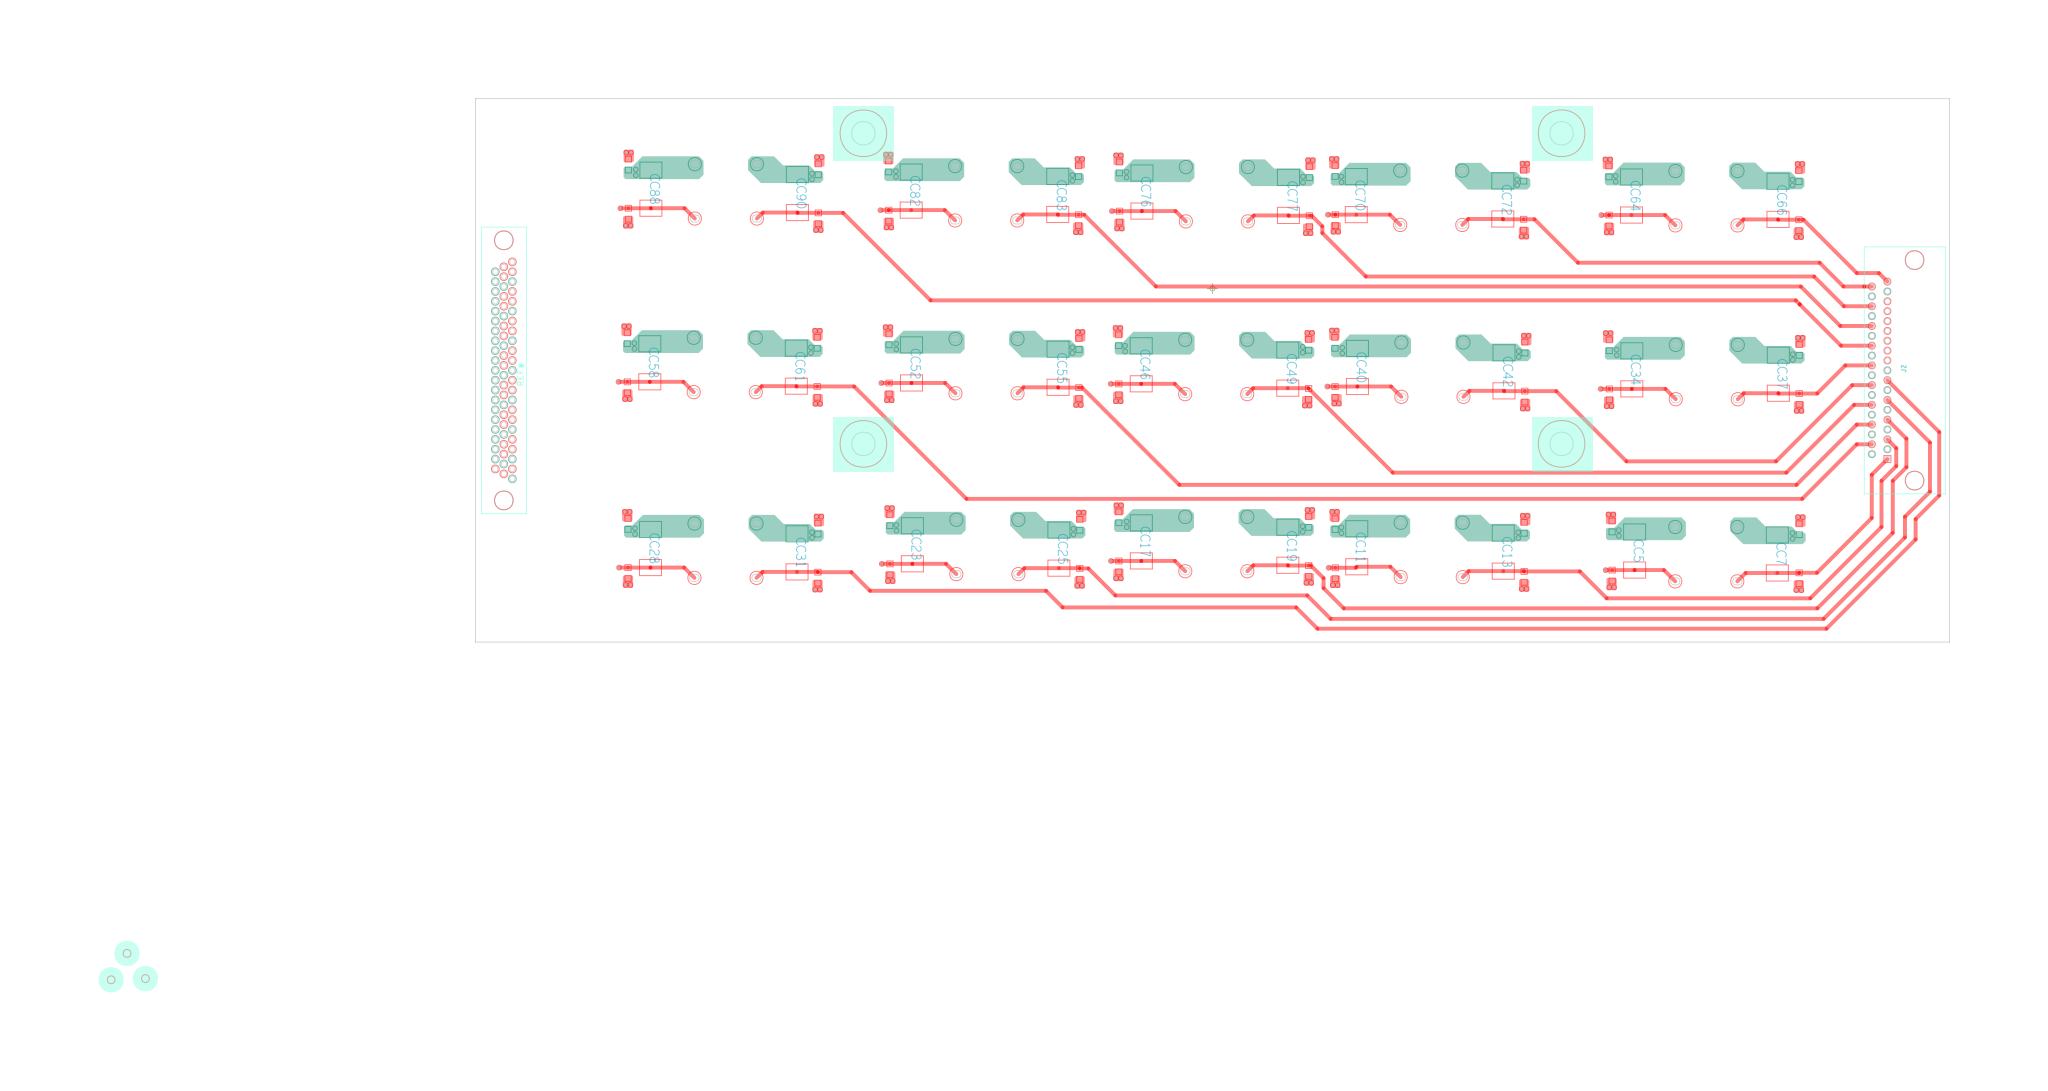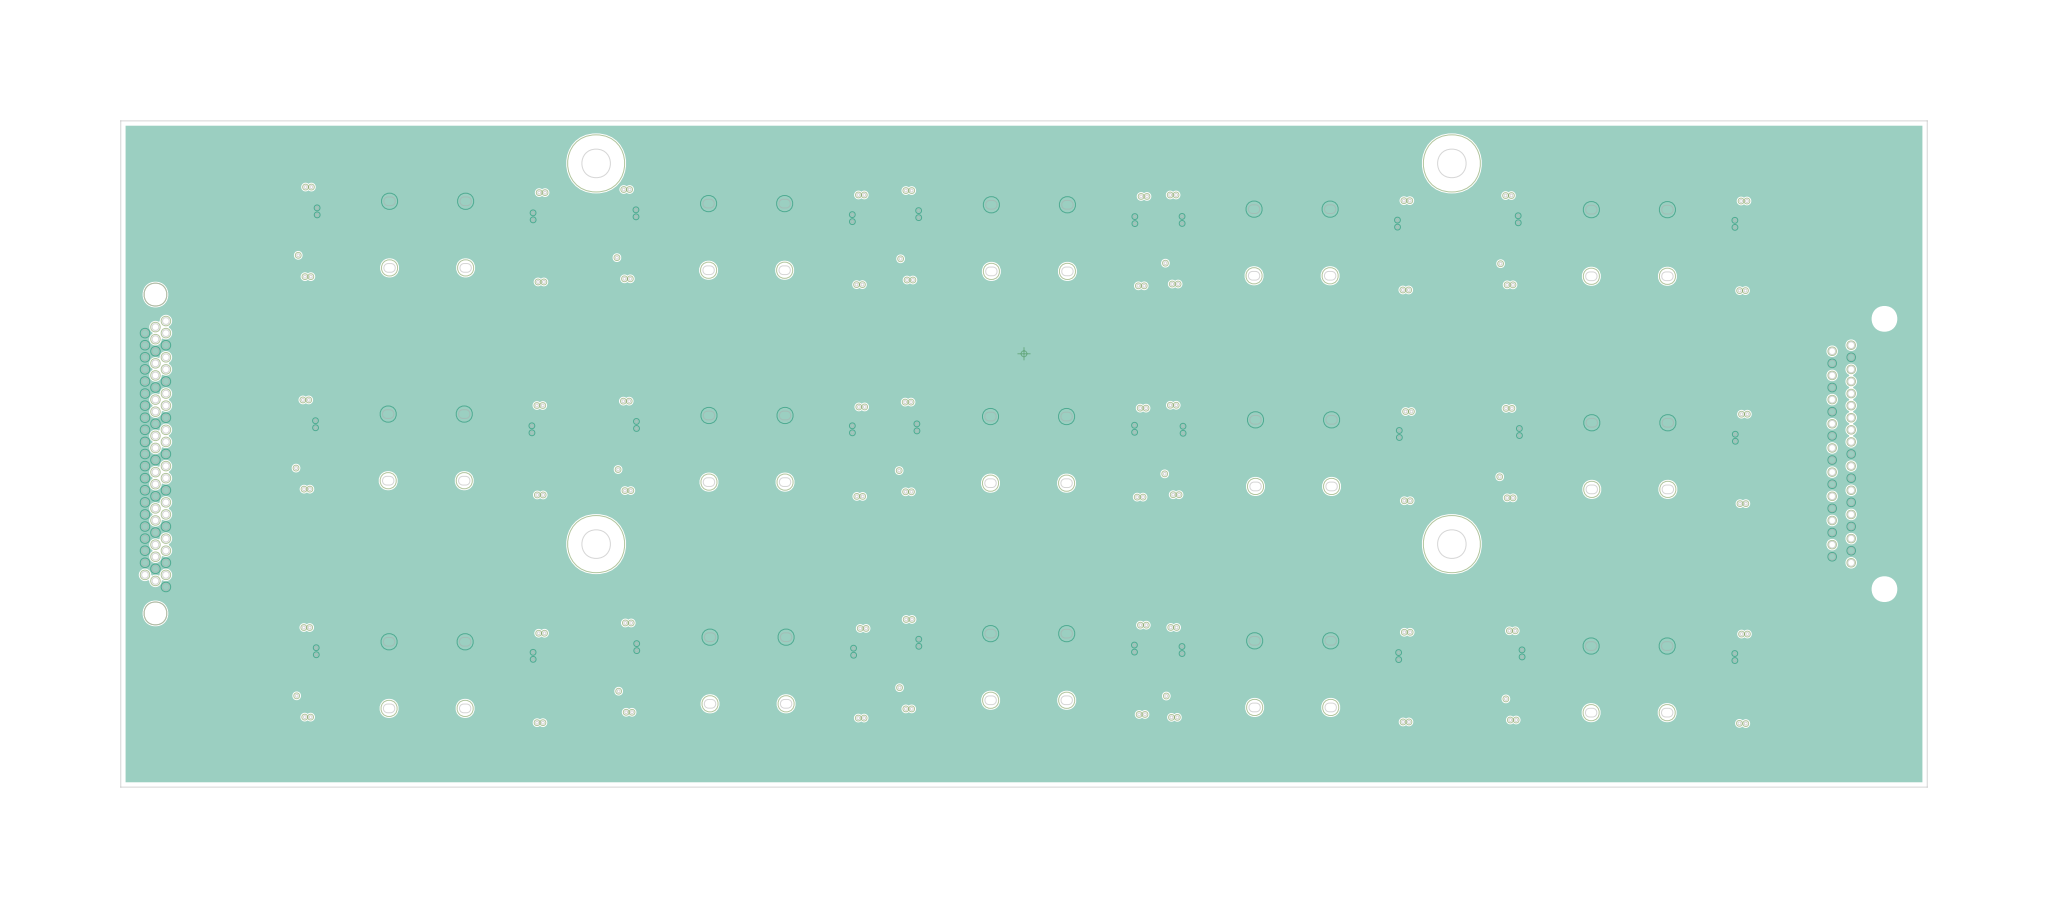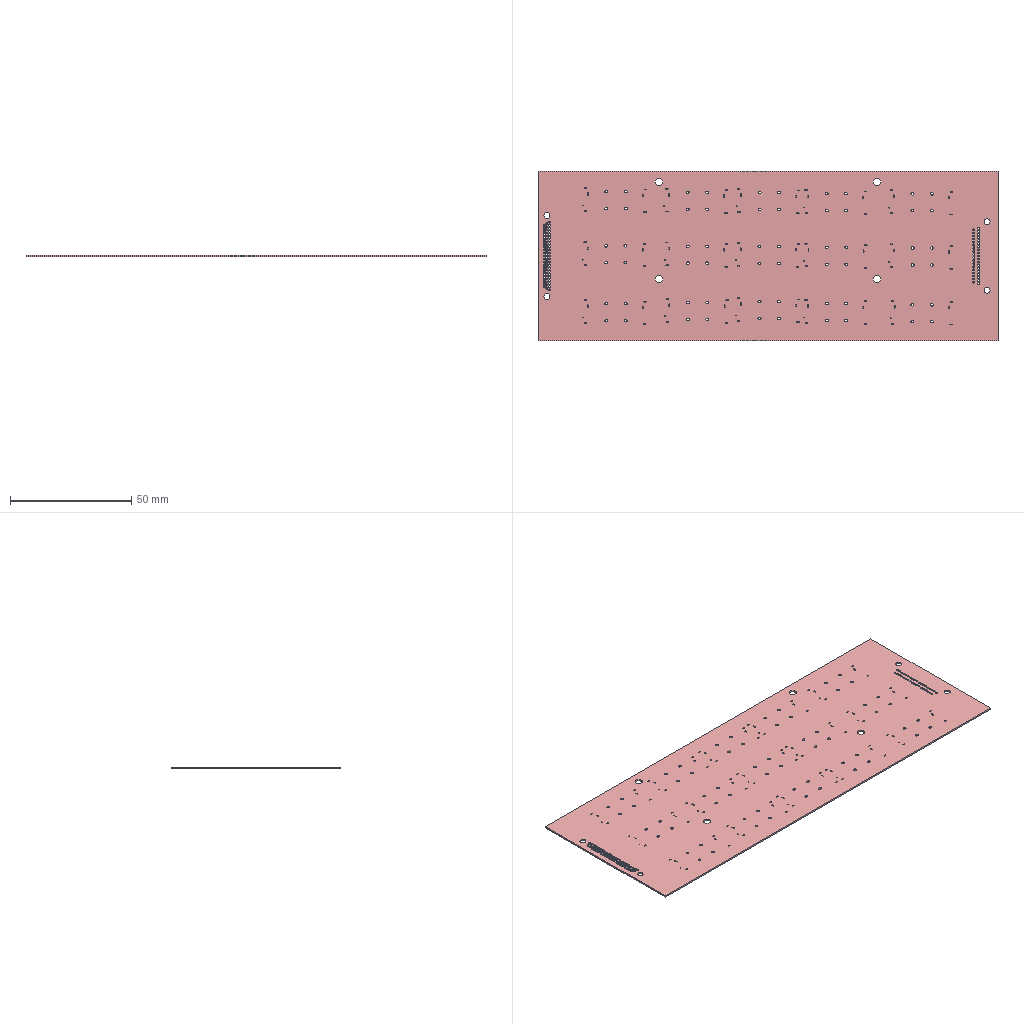Circuit board layout | Cadence Allegro | box 190 x 70 x 0.7 mm
Layer stack:
# Cadence Allegro layer stack of  (unit mm; from the constraint file cross-section; dielectric type: 0 not recorded (Allegro does not mark core vs prepreg), 3 surface material)
index,name,kind,layer,copper_thickness_mm,dielectric_type,dielectric_thickness_mm,dielectric_material,dielectric_constant
0,Top Surface,other,,,,,,
1,TOP,copper,TOP,0.0305,,,,
2,Dielectric1,dielectric,,,0,0.2032,FR-4,4.5
3,GND2,copper,GND2,0.0305,,,,
4,Dielectric2,dielectric,,,0,0.2032,FR-4,4.5
5,GND3,copper,GND3,0.0305,,,,
6,Dielectric3,dielectric,,,0,0.2032,FR-4,4.5
7,BOTTOM,copper,BOTTOM,0.0305,,,,
8,Bottom Surface,other,,,,,,
# drill layer pairs: low layer,high layer
drill_pair,TOP,BOTTOM
Part placement:
REFDES,COMP_VALUE,SYM_NAME,SYM_X,SYM_Y,SYM_ROTATE,SYM_MIRROR
CC4,1uF/50V,C0603,2027.992,-1206.161,270.000,NO
CC5,68uF/50V,C1812,2142.256,-1330.882,270.000,NO
CC6,1uF/50V,C0603,2028.386,-1455.201,270.000,NO
CC7,68uF/50V,C1812,2866.543,-1345.756,270.000,NO
CC8,1uF/50V,C0603,2977.339,-1468.843,270.000,NO
CC9,1uF/50V,C0603,2977.339,-1220.193,270.000,NO
CC10,1uF/50V,C0603,622.668,-1194.281,270.000,NO
CC11,68uF/50V,C1812,732.112,-1314.185,270.000,NO
CC12,1uF/50V,C0603,623.062,-1443.324,270.000,NO
CC13,68uF/50V,C1812,1475.683,-1336.287,270.000,NO
CC14,1uF/50V,C0603,1581.651,-1461.787,270.000,NO
CC15,1uF/50V,C0603,1581.651,-1213.138,270.000,NO
CC16,1uF/50V,C0603,-475.387,-1159.756,270.000,NO
CC17,68uF/50V,C1812,-361.123,-1284.480,270.000,NO
CC18,1uF/50V,C0603,-474.989,-1408.795,270.000,NO
CC19,68uF/50V,C1812,382.448,-1306.579,270.000,NO
CC20,1uF/50V,C0603,488.416,-1432.079,270.000,NO
CC21,1uF/50V,C0603,488.416,-1183.433,270.000,NO
CC22,1uF/50V,C0603,-1637.303,-1174.381,270.000,NO
CC23,68uF/50V,C1812,-1523.039,-1299.105,270.000,NO
CC24,1uF/50V,C0603,-1636.905,-1423.424,270.000,NO
CC25,68uF/50V,C1812,-779.468,-1321.208,270.000,NO
CC26,1uF/50V,C0603,-673.500,-1446.708,270.000,NO
CC27,1uF/50V,C0603,-673.500,-1198.058,270.000,NO
CC28,68uF/50V,C1812,-2852.026,-1318.119,270.000,NO
CC29,1uF/50V,C0603,-2966.290,-1193.394,270.000,NO
CC30,1uF/50V,C0603,-2965.893,-1442.434,270.000,NO
CC31,68uF/50V,C1812,-2108.456,-1340.217,270.000,NO
CC32,1uF/50V,C0603,-2002.487,-1465.717,270.000,NO
CC33,1uF/50V,C0603,-2002.487,-1217.072,270.000,NO
CC34,68uF/50V,C1812,2128.085,-412.123,270.000,NO
CC35,1uF/50V,C0603,2013.822,-287.399,270.000,NO
CC36,1uF/50V,C0603,2014.219,-536.438,270.000,NO
CC37,68uF/50V,C1812,2871.656,-434.222,270.000,NO
CC38,1uF/50V,C0603,2977.625,-559.722,270.000,NO
CC39,1uF/50V,C0603,2977.625,-311.076,270.000,NO
CC40,68uF/50V,C1812,735.685,-400.026,270.000,NO
CC41,1uF/50V,C0603,621.421,-275.302,270.000,NO
CC42,68uF/50V,C1812,1479.256,-422.129,270.000,NO
CC43,1uF/50V,C0603,621.819,-524.341,270.000,NO
CC44,1uF/50V,C0603,1585.224,-547.629,270.000,NO
CC45,1uF/50V,C0603,1585.224,-298.979,270.000,NO
CC46,68uF/50V,C1812,-361.637,-386.443,270.000,NO
CC47,1uF/50V,C0603,-475.900,-261.723,270.000,NO
CC48,1uF/50V,C0603,-475.507,-510.762,270.000,NO
CC49,68uF/50V,C1812,381.934,-408.546,270.000,NO
CC50,1uF/50V,C0603,487.903,-534.046,270.000,NO
CC51,1uF/50V,C0603,487.903,-285.396,270.000,NO
CC52,68uF/50V,C1812,-1527.421,-382.069,270.000,NO
CC53,1uF/50V,C0603,-1641.685,-257.345,270.000,NO
CC54,1uF/50V,C0603,-1641.291,-506.384,270.000,NO
CC55,68uF/50V,C1812,-783.850,-404.167,270.000,NO
CC56,1uF/50V,C0603,-677.882,-529.667,270.000,NO
CC57,1uF/50V,C0603,-677.882,-281.018,270.000,NO
CC58,68uF/50V,C1812,-2855.672,-376.217,270.000,NO
CC59,1uF/50V,C0603,-2969.935,-251.493,270.000,NO
CC60,1uF/50V,C0603,-2969.542,-500.532,270.000,NO
CC61,68uF/50V,C1812,-2112.101,-398.316,270.000,NO
CC62,1uF/50V,C0603,-2006.132,-523.816,270.000,NO
CC63,1uF/50V,C0603,-2006.132,-275.170,270.000,NO
CC64,68uF/50V,C1812,2126.329,469.317,270.000,NO
CC65,1uF/50V,C0603,2012.065,594.042,270.000,NO
CC66,68uF/50V,C1812,2869.900,447.219,270.000,NO
CC67,1uF/50V,C0603,2012.463,345.002,270.000,NO
CC68,1uF/50V,C0603,2975.868,321.719,270.000,NO
CC69,1uF/50V,C0603,2975.868,570.365,270.000,NO
CC70,68uF/50V,C1812,729.680,471.434,270.000,NO
CC71,1uF/50V,C0603,622.645,596.162,270.000,NO
CC72,68uF/50V,C1812,1473.255,449.335,270.000,NO
CC73,1uF/50V,C0603,623.042,347.123,270.000,NO
CC74,1uF/50V,C0603,1579.223,323.835,270.000,NO
CC75,1uF/50V,C0603,1579.223,572.481,270.000,NO
CC76,68uF/50V,C1812,-358.084,489.540,270.000,NO
CC77,68uF/50V,C1812,385.487,467.441,270.000,NO
CC78,1uF/50V,C0603,-472.348,614.264,270.000,NO
CC79,1uF/50V,C0603,-471.954,365.225,270.000,NO
CC80,1uF/50V,C0603,491.455,341.941,270.000,NO
CC81,1uF/50V,C0603,491.455,590.587,270.000,NO
CC82,68uF/50V,C1812,-1529.030,494.347,270.000,NO
CC83,68uF/50V,C1812,-785.455,472.249,270.000,NO
CC84,1uF/50V,C0603,-1643.294,619.072,270.000,NO
CC85,1uF/50V,C0603,-1642.896,370.032,270.000,NO
CC86,1uF/50V,C0603,-679.491,346.749,270.000,NO
CC87,1uF/50V,C0603,-679.491,595.399,270.000,NO
CC88,68uF/50V,C1812,-2850.054,503.991,270.000,NO
CC89,1uF/50V,C0603,-2964.318,628.715,270.000,NO
CC90,68uF/50V,C1812,-2106.483,481.888,270.000,NO
CC91,1uF/50V,C0603,-2963.924,379.676,270.000,NO
CC92,1uF/50V,C0603,-2000.515,356.388,270.000,NO
CC93,1uF/50V,C0603,-2000.515,605.038,270.000,NO
J1,J30JZPN66ZKNA000,J30JZ66,-3596.457,-414.622,90.000,NO
J2,J63A,J30JZLN37,3385.827,-414.622,90.000,NO
LC1,XRT16128B-122VFR1L,XRT16128B-122VFR1L,2505.850,-1346.756,270.000,NO
LC2,XRT16128B-122VFR1L,XRT16128B-122VFR1L,1112.581,-1325.232,270.000,NO
LC3,XRT16128B-122VFR1L,XRT16128B-122VFR1L,19.346,-1295.528,270.000,NO
LC4,XRT16128B-122VFR1L,XRT16128B-122VFR1L,-1142.571,-1310.152,270.000,NO
LC5,XRT16128B-122VFR1L,XRT16128B-122VFR1L,-2471.558,-1329.166,270.000,NO
LC6,XRT16128B-122VFR1L,XRT16128B-122VFR1L,2508.554,-423.171,270.000,NO
LC7,XRT16128B-122VFR1L,XRT16128B-122VFR1L,1116.154,-411.074,270.000,NO
LC8,XRT16128B-122VFR1L,XRT16128B-122VFR1L,18.832,-397.495,270.000,NO
LC9,XRT16128B-122VFR1L,XRT16128B-122VFR1L,-1146.953,-393.116,270.000,NO
LC10,XRT16128B-122VFR1L,XRT16128B-122VFR1L,-2475.203,-387.265,270.000,NO
LC11,XRT16128B-122VFR1L,XRT16128B-122VFR1L,2506.797,458.270,270.000,NO
LC12,XRT16128B-122VFR1L,XRT16128B-122VFR1L,1110.149,460.386,270.000,NO
LC13,XRT16128B-122VFR1L,XRT16128B-122VFR1L,22.381,478.493,270.000,NO
LC14,XRT16128B-122VFR1L,XRT16128B-122VFR1L,-1148.562,483.300,270.000,NO
LC15,XRT16128B-122VFR1L,XRT16128B-122VFR1L,-2469.586,492.943,270.000,NO
Pad and via stacks, first 115 of 279 lines:
# Allegro (Cadence) via spans and padstacks; design units: ("mils" 3 1000)
# via spans: padstack,start_layer,end_layer,net_example,count
VIA12X24,ETCH/TOP,ETCH/BOTTOM,V5,195
# Allegro padstack definitions: name,start_layer,end_layer,drill,plating,holeType,type
PAD19,"ETCH/TOP","ETCH/TOP",0.0,"NON_PLATED","none","smd"
PAD13,"ETCH/TOP","ETCH/TOP",0.0,"NON_PLATED","none","smd"
PAD12,"ETCH/TOP","ETCH/TOP",0.0,"NON_PLATED","none","smd"
PAD17,"ETCH/TOP","ETCH/TOP",0.0,"NON_PLATED","none","smd"
PAD15,"ETCH/TOP","ETCH/TOP",0.0,"NON_PLATED","none","smd"
PAD16,"ETCH/TOP","ETCH/TOP",0.0,"NON_PLATED","none","smd"
PAD1,"ETCH/TOP","ETCH/TOP",0.0,"NON_PLATED","none","smd"
PAD46,"ETCH/TOP","ETCH/TOP",0.0,"NON_PLATED","none","smd"
PAD44,"ETCH/TOP","ETCH/TOP",0.0,"NON_PLATED","none","smd"
PAD8,"ETCH/TOP","ETCH/TOP",0.0,"NON_PLATED","none","smd"
PAD5,"ETCH/TOP","ETCH/TOP",0.0,"NON_PLATED","none","smd"
PAD9,"ETCH/TOP","ETCH/TOP",0.0,"NON_PLATED","none","smd"
PAD10,"ETCH/TOP","ETCH/TOP",0.0,"NON_PLATED","none","smd"
PAD25,"ETCH/TOP","ETCH/TOP",0.0,"NON_PLATED","none","smd"
PAD4,"ETCH/TOP","ETCH/TOP",0.0,"NON_PLATED","none","smd"
PAD7,"ETCH/TOP","ETCH/TOP",0.0,"NON_PLATED","none","smd"
PAD6,"ETCH/TOP","ETCH/TOP",0.0,"NON_PLATED","none","smd"
PAD3,"ETCH/TOP","ETCH/TOP",0.0,"NON_PLATED","none","smd"
PAD31,"ETCH/TOP","ETCH/TOP",0.0,"NON_PLATED","none","smd"
PAD22,"ETCH/TOP","ETCH/TOP",0.0,"NON_PLATED","none","smd"
PAD41,"ETCH/TOP","ETCH/TOP",0.0,"NON_PLATED","none","smd"
PAD42,"ETCH/TOP","ETCH/TOP",0.0,"NON_PLATED","none","smd"
PAD43,"ETCH/TOP","ETCH/TOP",0.0,"NON_PLATED","none","smd"
PAD45,"ETCH/TOP","ETCH/TOP",0.0,"NON_PLATED","none","smd"
PAD2,"ETCH/TOP","ETCH/TOP",0.0,"NON_PLATED","none","smd"
PAD14,"ETCH/TOP","ETCH/TOP",0.0,"NON_PLATED","none","smd"
PAD21,"ETCH/TOP","ETCH/TOP",0.0,"NON_PLATED","none","smd"
PAD28,"ETCH/TOP","ETCH/TOP",0.0,"NON_PLATED","none","smd"
PAD26,"ETCH/TOP","ETCH/TOP",0.0,"NON_PLATED","none","smd"
PAD27,"ETCH/TOP","ETCH/TOP",0.0,"NON_PLATED","none","smd"
PAD18,"ETCH/TOP","ETCH/TOP",0.0,"NON_PLATED","none","smd"
PAD29,"ETCH/TOP","ETCH/TOP",0.0,"NON_PLATED","none","smd"
PAD20,"ETCH/TOP","ETCH/TOP",0.0,"NON_PLATED","none","smd"
PAD39,"ETCH/TOP","ETCH/TOP",0.0,"NON_PLATED","none","smd"
PAD40,"ETCH/TOP","ETCH/TOP",0.0,"NON_PLATED","none","smd"
PAD30,"ETCH/TOP","ETCH/TOP",0.0,"NON_PLATED","none","smd"
PAD48,"ETCH/TOP","ETCH/TOP",0.0,"NON_PLATED","none","smd"
PAD47,"ETCH/TOP","ETCH/TOP",0.0,"NON_PLATED","none","smd"
PAD49,"ETCH/TOP","ETCH/TOP",0.0,"NON_PLATED","none","smd"
PAD50,"ETCH/TOP","ETCH/TOP",0.0,"NON_PLATED","none","smd"
PAD53,"ETCH/TOP","ETCH/TOP",0.0,"NON_PLATED","none","smd"
F45,"ETCH/TOP","ETCH/TOP",0.0,"NON_PLATED","none","smd"
R88X76,"ETCH/TOP","ETCH/TOP",0.0,"PLATED","none","smd"
R127X121,"ETCH/TOP","ETCH/TOP",0.0,"PLATED","none","smd"
R127X152,"ETCH/TOP","ETCH/TOP",0.0,"NON_PLATED","none","smd"
R14X25,"ETCH/TOP","ETCH/TOP",0.0,"NON_PLATED","none","smd"
R165X317,"ETCH/TOP","ETCH/TOP",0.0,"NON_PLATED","none","smd"
R259X218,"ETCH/TOP","ETCH/TOP",0.0,"NON_PLATED","none","smd"
R70X22,"ETCH/TOP","ETCH/TOP",0.0,"NON_PLATED","none","smd"
R75X85,"ETCH/TOP","ETCH/TOP",0.0,"NON_PLATED","none","smd"
Y5,"ETCH/TOP","ETCH/TOP",0.0,"NON_PLATED","none","smd"
R16X30,"ETCH/TOP","ETCH/TOP",0.0,"NON_PLATED","none","smd"
F62X58,"ETCH/TOP","ETCH/TOP",0.0,"PLATED","none","smd"
R15X28,"ETCH/TOP","ETCH/TOP",0.0,"NON_PLATED","none","smd"
R195X280,"ETCH/TOP","ETCH/TOP",0.0,"NON_PLATED","none","smd"
R45X200,"ETCH/TOP","ETCH/TOP",0.0,"NON_PLATED","none","smd"
R50X30,"ETCH/TOP","ETCH/TOP",0.0,"NON_PLATED","none","smd"
R127X120,"ETCH/TOP","ETCH/TOP",0.0,"NON_PLATED","none","smd"
R31X24,"ETCH/TOP","ETCH/TOP",0.0,"NON_PLATED","none","smd"
R215X60,"ETCH/TOP","ETCH/TOP",0.0,"NON_PLATED","none","smd"
S17,"ETCH/TOP","ETCH/TOP",0.0,"NON_PLATED","none","smd"
R23X25,"ETCH/TOP","ETCH/TOP",0.0,"NON_PLATED","none","smd"
R19X32,"ETCH/TOP","ETCH/TOP",0.0,"NON_PLATED","none","smd"
R61X15,"ETCH/TOP","ETCH/TOP",0.0,"NON_PLATED","none","smd"
R45X150,"ETCH/TOP","ETCH/TOP",0.0,"NON_PLATED","none","smd"
R12X8,"ETCH/TOP","ETCH/TOP",0.0,"NON_PLATED","none","smd"
R91X127,"ETCH/TOP","ETCH/TOP",0.0,"NON_PLATED","none","smd"
S91,"ETCH/TOP","ETCH/TOP",0.0,"NON_PLATED","none","smd"
R55X99,"ETCH/TOP","ETCH/TOP",0.0,"NON_PLATED","none","smd"
R299X199,"ETCH/TOP","ETCH/TOP",0.0,"NON_PLATED","none","smd"
R114X165,"ETCH/TOP","ETCH/TOP",0.0,"NON_PLATED","none","smd"
R60X90,"ETCH/TOP","ETCH/TOP",0.0,"NON_PLATED","none","smd"
R6X10,"ETCH/TOP","ETCH/TOP",0.0,"NON_PLATED","none","smd"
Y10,"ETCH/TOP","ETCH/TOP",0.0,"NON_PLATED","none","smd"
R114X74,"ETCH/TOP","ETCH/TOP",0.0,"NON_PLATED","none","smd"
R30X130,"ETCH/TOP","ETCH/TOP",0.0,"PLATED","none","smd"
R50X127,"ETCH/TOP","ETCH/TOP",0.0,"NON_PLATED","none","smd"
R18X20,"ETCH/TOP","ETCH/TOP",0.0,"NON_PLATED","none","smd"
R60X71,"ETCH/TOP","ETCH/TOP",0.0,"NON_PLATED","none","smd"
R48X71,"ETCH/TOP","ETCH/TOP",0.0,"NON_PLATED","none","smd"
R80X30,"ETCH/TOP","ETCH/TOP",0.0,"PLATED","none","smd"
FLASH_0,"ETCH/TOP","ETCH/TOP",0.0,"PLATED","none","smd"
Y3,"ETCH/TOP","ETCH/TOP",0.0,"PLATED","none","smd"
R170X25,"ETCH/TOP","ETCH/TOP",0.0,"PLATED","none","smd"
R70X25,"ETCH/TOP","ETCH/TOP",0.0,"PLATED","none","smd"
R43X14,"ETCH/TOP","ETCH/TOP",0.0,"PLATED","none","smd"
R33X10,"ETCH/TOP","ETCH/TOP",0.0,"PLATED","none","smd"
R636X23,"ETCH/TOP","ETCH/TOP",0.0,"PLATED","none","smd"
R155X35,"ETCH/TOP","ETCH/TOP",0.0,"PLATED","none","smd"
R60X20,"ETCH/TOP","ETCH/TOP",0.0,"PLATED","none","smd"
R120X70,"ETCH/TOP","ETCH/TOP",0.0,"PLATED","none","smd"
SMD0_45R,"ETCH/TOP","ETCH/TOP",0.0,"PLATED","none","smd"
Y42,"ETCH/TOP","ETCH/TOP",0.0,"PLATED","none","smd"
R85X65,"ETCH/TOP","ETCH/TOP",0.0,"PLATED","none","smd"
Y30,"ETCH/TOP","ETCH/TOP",0.0,"PLATED","none","smd"
R53X20,"ETCH/TOP","ETCH/TOP",0.0,"PLATED","none","smd"
R55X40,"ETCH/TOP","ETCH/TOP",0.0,"PLATED","none","smd"
R155X25,"ETCH/TOP","ETCH/TOP",0.0,"PLATED","none","smd"
F17X17,"ETCH/TOP","ETCH/TOP",0.0,"PLATED","none","smd"
F89X32,"ETCH/TOP","ETCH/TOP",0.0,"PLATED","none","smd"
R8X2,"ETCH/TOP","ETCH/TOP",0.0,"PLATED","none","smd"
SMD40X20,"ETCH/TOP","ETCH/TOP",0.0,"PLATED","none","smd"
R340X185,"ETCH/TOP","ETCH/TOP",0.0,"PLATED","none","smd"
R27X10,"ETCH/TOP","ETCH/TOP",0.0,"PLATED","none","smd"
R22X11,"ETCH/TOP","ETCH/TOP",0.0,"PLATED","none","smd"
R32X36,"ETCH/TOP","ETCH/TOP",0.0,"PLATED","none","smd"
S21X20,"ETCH/TOP","ETCH/TOP",0.0,"PLATED","none","smd"
R13X10,"ETCH/TOP","ETCH/TOP",0.0,"PLATED","none","smd"
R75X28,"ETCH/TOP","ETCH/TOP",0.0,"PLATED","none","smd"
R25X15,"ETCH/TOP","ETCH/TOP",0.0,"NON_PLATED","none","smd"
C0_5,"ETCH/TOP","ETCH/TOP",0.0,"PLATED","none","smd"
Design rules, without the lines most boards share, first 14 of 31 lines:
# Cadence Allegro design rules of  (from the Constraint Manager export constraints.dcfx, design unit mil; typed fields in mm)
# columns: name | kind | enabled | priority | scope1 | scope2 | descriptor | typed fields (field=value)
# Allegro precedence (priority 1 wins): 1 Region class-to-class, 2 Region class, 3 Region, 4 class-to-class, 5 DiffPair/Bus/NetGroup override, 6 NetClass, 7 constraint set (CSet) default
# per-layer values are written LAYER=value in the descriptor and LAYER:mm in the typed field; a maximum of 0 means no limit set
# --- net classes (and buses / net groups) ---
PHY_R | NetClass | enabled | 6 | no members | All | Net Class (members: 0) |
PHY_T | NetClass | enabled | 6 | no members | All | Net Class (members: 0) |
DDR3_A | NetClass | enabled | 6 | no members | All | Net Class (members: 0) |
DDR3_DQH1 | NetClass | enabled | 6 | no members | All | Net Class (members: 0) |
DDR3_DQL1 | NetClass | enabled | 6 | no members | All | Net Class (members: 0) |
DDR3_DQH0 | NetClass | enabled | 6 | no members | All | Net Class (members: 0) |
DDR3_DQL0 | NetClass | enabled | 6 | no members | All | Net Class (members: 0) |
# --- track widths, neck and differential-pair gap (physical constraint sets) ---
DEFAULT | PhysicalCSet | enabled | 7 | Design default | All | Physical Constraint (Min Line Width=6mil) (Max Line Width=0mil) (Min Neck Width=6mil) (Max Neck Length=0mil) (DiffPair Primary Gap=6mil) (DiffPair Neck Gap=0mil) (DiffPair Min Space=0mil) (DiffPair Coupled +Tol=0mil) (DiffPair Coupled -Tol=0mil) (Min BB Via Stagger=5mil) (Max BB Via Stagger=0mil) (T-junctions=ANYWHERE) (Pad-pad direct connect=ALL_ALLOWED) (Allowed vias=VIA12X24) | diffp_coupled_plus=0 diffp_coupled_minus=0 diffp_primary_gap=0.1524 min_line_width=0.1524 diffp_neck_gap=0 min_neck_width=0.1524 max_line_width=0 maximum_neck_length=0 diffp_min_space=0 min_bvia_stagger=0.127 max_bvia_stagger=0 pad_pad_direct_connect=ALL_ALLOWED allow_on_etch_subclass=TRUE ts_allowed=ANYWHERE vias=VIA12X24